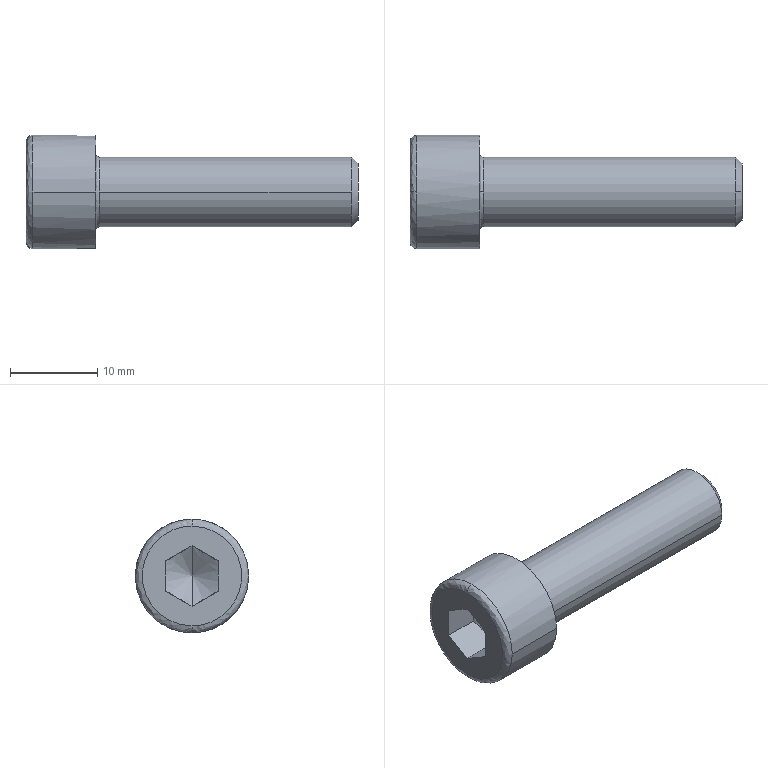Part | STEP file | Broached Socket Head Cap Screw - Metric M8x1.25 x 30 | 1 solid | 21 faces | box 38 x 13 x 13 mm | volume 2409 mm3 | plane 9 | spline 4 | cylinder 4 | cone 4 | commonest cylinder face diameters 8 x2 13 x2